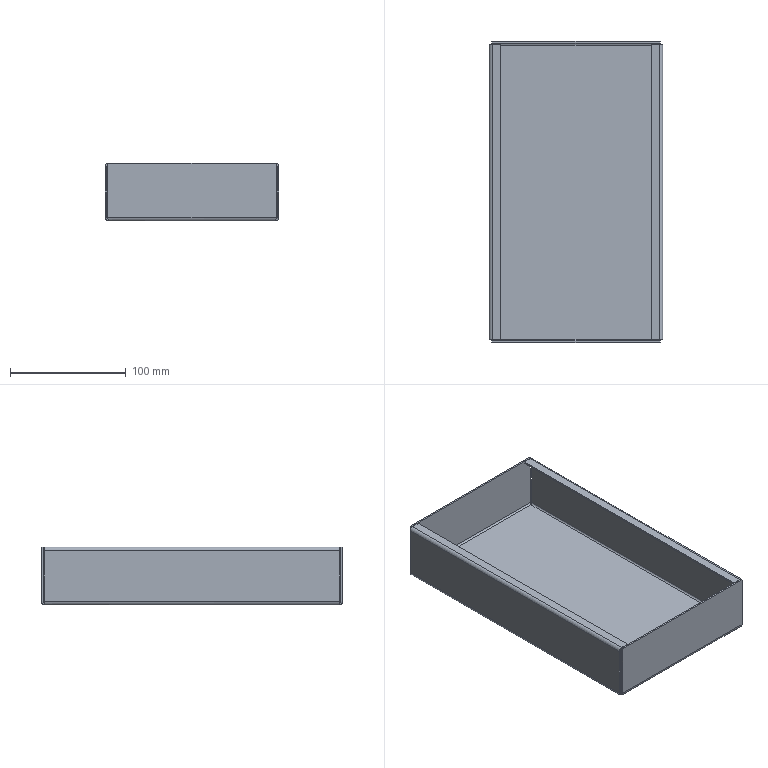Part | STEP file | Dial wheel cover SGN-5-09 | 1 solid | 54 faces | box 150 x 260 x 50 mm | volume 121443 mm3 | plane 34 | cylinder 12 | spline 8 | commonest cylinder face diameters 3 x6 6 x6